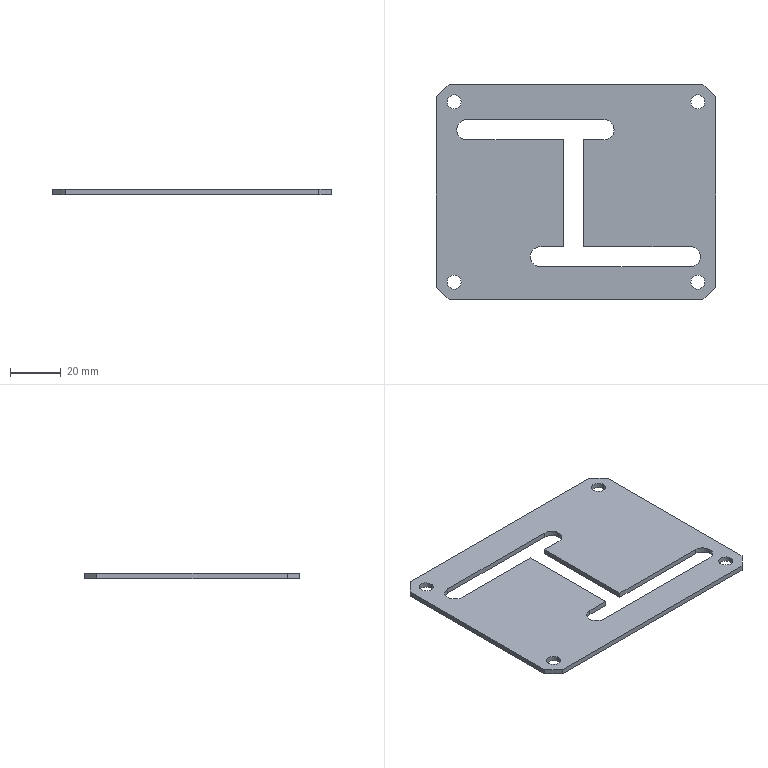Part | SolidWorks | features Cut 2, Extrusion 1 | 1 solid | 32 faces | box 110 x 85 x 2 mm | volume 15729 mm3 | plane 18 | cylinder 14 | commonest cylinder face diameters 5.5 x8 8 x5 8.02 x1
STEP:
#1=CARTESIAN_POINT('',(356.25,122.427,0.));
#2=VERTEX_POINT('',#1);
#3=CARTESIAN_POINT('',(361.75,122.427,0.));
#4=VERTEX_POINT('',#3);
#5=CARTESIAN_POINT('',(359.,122.427,0.));
#6=DIRECTION('',(0.,0.,1.));
#7=DIRECTION('',(1.,0.,0.));
#8=AXIS2_PLACEMENT_3D('',#5,#6,#7);
#9=CIRCLE('',#8,2.75);
#10=EDGE_CURVE('',#2,#4,#9,.T.);
#11=ORIENTED_EDGE('',*,*,#10,.F.);
#12=CARTESIAN_POINT('',(356.25,122.427,2.));
#13=VERTEX_POINT('',#12);
#14=CARTESIAN_POINT('',(356.25,122.427,0.));
#15=DIRECTION('',(0.,0.,1.));
#16=VECTOR('',#15,1000.);
#17=LINE('',#14,#16);
#18=EDGE_CURVE('',#2,#13,#17,.T.);
#19=ORIENTED_EDGE('',*,*,#18,.T.);
#20=CARTESIAN_POINT('',(361.75,122.427,2.));
#21=VERTEX_POINT('',#20);
#22=CARTESIAN_POINT('',(359.,122.427,2.));
#23=DIRECTION('',(0.,0.,1.));
#24=DIRECTION('',(1.,0.,0.));
#25=AXIS2_PLACEMENT_3D('',#22,#23,#24);
#26=CIRCLE('',#25,2.75);
#27=EDGE_CURVE('',#13,#21,#26,.T.);
#28=ORIENTED_EDGE('',*,*,#27,.T.);
#29=CARTESIAN_POINT('',(361.75,122.427,0.));
#30=DIRECTION('',(0.,0.,1.));
#31=VECTOR('',#30,1000.);
#32=LINE('',#29,#31);
#33=EDGE_CURVE('',#4,#21,#32,.T.);
#34=ORIENTED_EDGE('',*,*,#33,.F.);
#35=EDGE_LOOP('',(#11,#19,#28,#34));
#36=FACE_OUTER_BOUND('',#35,.T.);
#37=CARTESIAN_POINT('',(359.,122.427,0.));
#38=DIRECTION('',(0.,0.,1.));
#39=DIRECTION('',(1.,0.,0.));
#40=AXIS2_PLACEMENT_3D('',#37,#38,#39);
#41=CYLINDRICAL_SURFACE('',#40,2.75);
#42=ADVANCED_FACE('',(#36),#41,.F.);
#43=CARTESIAN_POINT('',(452.25,122.427,0.));
#44=VERTEX_POINT('',#43);
#45=CARTESIAN_POINT('',(457.75,122.427,0.));
#46=VERTEX_POINT('',#45);
#47=CARTESIAN_POINT('',(455.,122.427,0.));
#48=DIRECTION('',(0.,0.,1.));
#49=DIRECTION('',(1.,0.,0.));
#50=AXIS2_PLACEMENT_3D('',#47,#48,#49);
#51=CIRCLE('',#50,2.75);
#52=EDGE_CURVE('',#44,#46,#51,.T.);
#53=ORIENTED_EDGE('',*,*,#52,.F.);
#54=CARTESIAN_POINT('',(452.25,122.427,2.));
#55=VERTEX_POINT('',#54);
#56=CARTESIAN_POINT('',(452.25,122.427,0.));
#57=DIRECTION('',(0.,0.,1.));
#58=VECTOR('',#57,1000.);
#59=LINE('',#56,#58);
#60=EDGE_CURVE('',#44,#55,#59,.T.);
#61=ORIENTED_EDGE('',*,*,#60,.T.);
#62=CARTESIAN_POINT('',(457.75,122.427,2.));
#63=VERTEX_POINT('',#62);
#64=CARTESIAN_POINT('',(455.,122.427,2.));
#65=DIRECTION('',(0.,0.,1.));
#66=DIRECTION('',(1.,0.,0.));
#67=AXIS2_PLACEMENT_3D('',#64,#65,#66);
#68=CIRCLE('',#67,2.75);
#69=EDGE_CURVE('',#55,#63,#68,.T.);
#70=ORIENTED_EDGE('',*,*,#69,.T.);
#71=CARTESIAN_POINT('',(457.75,122.427,0.));
#72=DIRECTION('',(0.,0.,1.));
#73=VECTOR('',#72,1000.);
#74=LINE('',#71,#73);
#75=EDGE_CURVE('',#46,#63,#74,.T.);
#76=ORIENTED_EDGE('',*,*,#75,.F.);
#77=EDGE_LOOP('',(#53,#61,#70,#76));
#78=FACE_OUTER_BOUND('',#77,.T.);
#79=CARTESIAN_POINT('',(455.,122.427,0.));
#80=DIRECTION('',(0.,0.,1.));
#81=DIRECTION('',(1.,0.,0.));
#82=AXIS2_PLACEMENT_3D('',#79,#80,#81);
#83=CYLINDRICAL_SURFACE('',#82,2.75);
#84=ADVANCED_FACE('',(#78),#83,.F.);
#85=CARTESIAN_POINT('',(356.25,51.427,0.));
#86=VERTEX_POINT('',#85);
#87=CARTESIAN_POINT('',(361.75,51.427,0.));
#88=VERTEX_POINT('',#87);
#89=CARTESIAN_POINT('',(359.,51.427,0.));
#90=DIRECTION('',(0.,0.,1.));
#91=DIRECTION('',(1.,0.,0.));
#92=AXIS2_PLACEMENT_3D('',#89,#90,#91);
#93=CIRCLE('',#92,2.75);
#94=EDGE_CURVE('',#86,#88,#93,.T.);
#95=ORIENTED_EDGE('',*,*,#94,.F.);
#96=CARTESIAN_POINT('',(356.25,51.427,2.));
#97=VERTEX_POINT('',#96);
#98=CARTESIAN_POINT('',(356.25,51.427,0.));
#99=DIRECTION('',(0.,0.,1.));
#100=VECTOR('',#99,1000.);
#101=LINE('',#98,#100);
#102=EDGE_CURVE('',#86,#97,#101,.T.);
#103=ORIENTED_EDGE('',*,*,#102,.T.);
#104=CARTESIAN_POINT('',(361.75,51.427,2.));
#105=VERTEX_POINT('',#104);
#106=CARTESIAN_POINT('',(359.,51.427,2.));
#107=DIRECTION('',(0.,0.,1.));
#108=DIRECTION('',(1.,0.,0.));
#109=AXIS2_PLACEMENT_3D('',#106,#107,#108);
#110=CIRCLE('',#109,2.75);
#111=EDGE_CURVE('',#97,#105,#110,.T.);
#112=ORIENTED_EDGE('',*,*,#111,.T.);
#113=CARTESIAN_POINT('',(361.75,51.427,0.));
#114=DIRECTION('',(0.,0.,1.));
#115=VECTOR('',#114,1000.);
#116=LINE('',#113,#115);
#117=EDGE_CURVE('',#88,#105,#116,.T.);
#118=ORIENTED_EDGE('',*,*,#117,.F.);
#119=EDGE_LOOP('',(#95,#103,#112,#118));
#120=FACE_OUTER_BOUND('',#119,.T.);
#121=CARTESIAN_POINT('',(359.,51.427,0.));
#122=DIRECTION('',(0.,0.,1.));
#123=DIRECTION('',(1.,0.,0.));
#124=AXIS2_PLACEMENT_3D('',#121,#122,#123);
#125=CYLINDRICAL_SURFACE('',#124,2.75);
#126=ADVANCED_FACE('',(#120),#125,.F.);
#127=CARTESIAN_POINT('',(452.25,51.427,0.));
#128=VERTEX_POINT('',#127);
#129=CARTESIAN_POINT('',(457.75,51.427,0.));
#130=VERTEX_POINT('',#129);
#131=CARTESIAN_POINT('',(455.,51.427,0.));
#132=DIRECTION('',(0.,0.,1.));
#133=DIRECTION('',(1.,0.,0.));
#134=AXIS2_PLACEMENT_3D('',#131,#132,#133);
#135=CIRCLE('',#134,2.75);
#136=EDGE_CURVE('',#128,#130,#135,.T.);
#137=ORIENTED_EDGE('',*,*,#136,.F.);
#138=CARTESIAN_POINT('',(452.25,51.427,2.));
#139=VERTEX_POINT('',#138);
#140=CARTESIAN_POINT('',(452.25,51.427,0.));
#141=DIRECTION('',(0.,0.,1.));
#142=VECTOR('',#141,1000.);
#143=LINE('',#140,#142);
#144=EDGE_CURVE('',#128,#139,#143,.T.);
#145=ORIENTED_EDGE('',*,*,#144,.T.);
#146=CARTESIAN_POINT('',(457.75,51.427,2.));
#147=VERTEX_POINT('',#146);
#148=CARTESIAN_POINT('',(455.,51.427,2.));
#149=DIRECTION('',(0.,0.,1.));
#150=DIRECTION('',(1.,0.,0.));
#151=AXIS2_PLACEMENT_3D('',#148,#149,#150);
#152=CIRCLE('',#151,2.75);
#153=EDGE_CURVE('',#139,#147,#152,.T.);
#154=ORIENTED_EDGE('',*,*,#153,.T.);
#155=CARTESIAN_POINT('',(457.75,51.427,0.));
#156=DIRECTION('',(0.,0.,1.));
#157=VECTOR('',#156,1000.);
#158=LINE('',#155,#157);
#159=EDGE_CURVE('',#130,#147,#158,.T.);
#160=ORIENTED_EDGE('',*,*,#159,.F.);
#161=EDGE_LOOP('',(#137,#145,#154,#160));
#162=FACE_OUTER_BOUND('',#161,.T.);
#163=CARTESIAN_POINT('',(455.,51.427,0.));
#164=DIRECTION('',(0.,0.,1.));
#165=DIRECTION('',(1.,0.,0.));
#166=AXIS2_PLACEMENT_3D('',#163,#164,#165);
#167=CYLINDRICAL_SURFACE('',#166,2.75);
#168=ADVANCED_FACE('',(#162),#167,.F.);
#169=CARTESIAN_POINT('',(422.,111.427,0.));
#170=VERTEX_POINT('',#169);
#171=CARTESIAN_POINT('',(418.,115.427,0.));
#172=VERTEX_POINT('',#171);
#173=CARTESIAN_POINT('',(418.,111.427,0.));
#174=DIRECTION('',(0.,0.,1.));
#175=DIRECTION('',(1.,0.,0.));
#176=AXIS2_PLACEMENT_3D('',#173,#174,#175);
#177=CIRCLE('',#176,4.);
#178=EDGE_CURVE('',#170,#172,#177,.T.);
#179=ORIENTED_EDGE('',*,*,#178,.F.);
#180=CARTESIAN_POINT('',(422.,111.427,2.));
#181=VERTEX_POINT('',#180);
#182=CARTESIAN_POINT('',(422.,111.427,0.));
#183=DIRECTION('',(0.,0.,1.));
#184=VECTOR('',#183,1000.);
#185=LINE('',#182,#184);
#186=EDGE_CURVE('',#170,#181,#185,.T.);
#187=ORIENTED_EDGE('',*,*,#186,.T.);
#188=CARTESIAN_POINT('',(418.,115.427,2.));
#189=VERTEX_POINT('',#188);
#190=CARTESIAN_POINT('',(418.,111.427,2.));
#191=DIRECTION('',(0.,0.,1.));
#192=DIRECTION('',(1.,0.,0.));
#193=AXIS2_PLACEMENT_3D('',#190,#191,#192);
#194=CIRCLE('',#193,4.);
#195=EDGE_CURVE('',#181,#189,#194,.T.);
#196=ORIENTED_EDGE('',*,*,#195,.T.);
#197=CARTESIAN_POINT('',(418.,115.427,0.));
#198=DIRECTION('',(0.,0.,1.));
#199=VECTOR('',#198,1000.);
#200=LINE('',#197,#199);
#201=EDGE_CURVE('',#172,#189,#200,.T.);
#202=ORIENTED_EDGE('',*,*,#201,.F.);
#203=EDGE_LOOP('',(#179,#187,#196,#202));
#204=FACE_OUTER_BOUND('',#203,.T.);
#205=CARTESIAN_POINT('',(418.,111.427,0.));
#206=DIRECTION('',(0.,0.,1.));
#207=DIRECTION('',(1.,0.,0.));
#208=AXIS2_PLACEMENT_3D('',#205,#206,#207);
#209=CYLINDRICAL_SURFACE('',#208,4.);
#210=ADVANCED_FACE('',(#204),#209,.F.);
#211=CARTESIAN_POINT('',(456.,61.427,0.));
#212=VERTEX_POINT('',#211);
#213=CARTESIAN_POINT('',(452.,65.427,0.));
#214=VERTEX_POINT('',#213);
#215=CARTESIAN_POINT('',(452.,61.427,0.));
#216=DIRECTION('',(0.,0.,1.));
#217=DIRECTION('',(1.,0.,0.));
#218=AXIS2_PLACEMENT_3D('',#215,#216,#217);
#219=CIRCLE('',#218,4.);
#220=EDGE_CURVE('',#212,#214,#219,.T.);
#221=ORIENTED_EDGE('',*,*,#220,.F.);
#222=CARTESIAN_POINT('',(456.,61.427,2.));
#223=VERTEX_POINT('',#222);
#224=CARTESIAN_POINT('',(456.,61.427,0.));
#225=DIRECTION('',(0.,0.,1.));
#226=VECTOR('',#225,1000.);
#227=LINE('',#224,#226);
#228=EDGE_CURVE('',#212,#223,#227,.T.);
#229=ORIENTED_EDGE('',*,*,#228,.T.);
#230=CARTESIAN_POINT('',(452.,65.427,2.));
#231=VERTEX_POINT('',#230);
#232=CARTESIAN_POINT('',(452.,61.427,2.));
#233=DIRECTION('',(0.,0.,1.));
#234=DIRECTION('',(1.,0.,0.));
#235=AXIS2_PLACEMENT_3D('',#232,#233,#234);
#236=CIRCLE('',#235,4.);
#237=EDGE_CURVE('',#223,#231,#236,.T.);
#238=ORIENTED_EDGE('',*,*,#237,.T.);
#239=CARTESIAN_POINT('',(452.,65.427,0.));
#240=DIRECTION('',(0.,0.,1.));
#241=VECTOR('',#240,1000.);
#242=LINE('',#239,#241);
#243=EDGE_CURVE('',#214,#231,#242,.T.);
#244=ORIENTED_EDGE('',*,*,#243,.F.);
#245=EDGE_LOOP('',(#221,#229,#238,#244));
#246=FACE_OUTER_BOUND('',#245,.T.);
#247=CARTESIAN_POINT('',(452.,61.427,0.));
#248=DIRECTION('',(0.,0.,1.));
#249=DIRECTION('',(1.,0.,0.));
#250=AXIS2_PLACEMENT_3D('',#247,#248,#249);
#251=CYLINDRICAL_SURFACE('',#250,4.);
#252=ADVANCED_FACE('',(#246),#251,.F.);
#253=CARTESIAN_POINT('',(352.,49.427,0.));
#254=VERTEX_POINT('',#253);
#255=CARTESIAN_POINT('',(357.,44.427,0.));
#256=VERTEX_POINT('',#255);
#257=CARTESIAN_POINT('',(352.,49.427,0.));
#258=DIRECTION('',(0.7071,-0.7071,0.));
#259=VECTOR('',#258,1000.);
#260=LINE('',#257,#259);
#261=EDGE_CURVE('',#254,#256,#260,.T.);
#262=ORIENTED_EDGE('',*,*,#261,.T.);
#263=CARTESIAN_POINT('',(357.,44.427,2.));
#264=VERTEX_POINT('',#263);
#265=CARTESIAN_POINT('',(357.,44.427,2.));
#266=DIRECTION('',(0.,0.,-1.));
#267=VECTOR('',#266,1000.);
#268=LINE('',#265,#267);
#269=EDGE_CURVE('',#264,#256,#268,.T.);
#270=ORIENTED_EDGE('',*,*,#269,.F.);
#271=CARTESIAN_POINT('',(352.,49.427,2.));
#272=VERTEX_POINT('',#271);
#273=CARTESIAN_POINT('',(352.,49.427,2.));
#274=DIRECTION('',(0.7071,-0.7071,0.));
#275=VECTOR('',#274,1000.);
#276=LINE('',#273,#275);
#277=EDGE_CURVE('',#272,#264,#276,.T.);
#278=ORIENTED_EDGE('',*,*,#277,.F.);
#279=CARTESIAN_POINT('',(352.,49.427,2.));
#280=DIRECTION('',(0.,0.,-1.));
#281=VECTOR('',#280,1000.);
#282=LINE('',#279,#281);
#283=EDGE_CURVE('',#272,#254,#282,.T.);
#284=ORIENTED_EDGE('',*,*,#283,.T.);
#285=EDGE_LOOP('',(#262,#270,#278,#284));
#286=FACE_OUTER_BOUND('',#285,.T.);
#287=CARTESIAN_POINT('',(352.,49.427,2.));
#288=DIRECTION('',(0.7071,0.7071,0.));
#289=DIRECTION('',(-0.7071,0.7071,0.));
#290=AXIS2_PLACEMENT_3D('',#287,#288,#289);
#291=PLANE('',#290);
#292=ADVANCED_FACE('',(#286),#291,.F.);
#293=CARTESIAN_POINT('',(457.,44.427,0.));
#294=VERTEX_POINT('',#293);
#295=CARTESIAN_POINT('',(357.,44.427,0.));
#296=DIRECTION('',(1.,0.,0.));
#297=VECTOR('',#296,1000.);
#298=LINE('',#295,#297);
#299=EDGE_CURVE('',#256,#294,#298,.T.);
#300=ORIENTED_EDGE('',*,*,#299,.T.);
#301=CARTESIAN_POINT('',(457.,44.427,2.));
#302=VERTEX_POINT('',#301);
#303=CARTESIAN_POINT('',(457.,44.427,2.));
#304=DIRECTION('',(0.,0.,-1.));
#305=VECTOR('',#304,1000.);
#306=LINE('',#303,#305);
#307=EDGE_CURVE('',#302,#294,#306,.T.);
#308=ORIENTED_EDGE('',*,*,#307,.F.);
#309=CARTESIAN_POINT('',(357.,44.427,2.));
#310=DIRECTION('',(1.,0.,0.));
#311=VECTOR('',#310,1000.);
#312=LINE('',#309,#311);
#313=EDGE_CURVE('',#264,#302,#312,.T.);
#314=ORIENTED_EDGE('',*,*,#313,.F.);
#315=ORIENTED_EDGE('',*,*,#269,.T.);
#316=EDGE_LOOP('',(#300,#308,#314,#315));
#317=FACE_OUTER_BOUND('',#316,.T.);
#318=CARTESIAN_POINT('',(357.,44.427,2.));
#319=DIRECTION('',(0.,1.,0.));
#320=DIRECTION('',(-1.,0.,0.));
#321=AXIS2_PLACEMENT_3D('',#318,#319,#320);
#322=PLANE('',#321);
#323=ADVANCED_FACE('',(#317),#322,.F.);
#324=CARTESIAN_POINT('',(462.,49.427,0.));
#325=VERTEX_POINT('',#324);
#326=CARTESIAN_POINT('',(457.,44.427,0.));
#327=DIRECTION('',(0.7071,0.7071,0.));
#328=VECTOR('',#327,1000.);
#329=LINE('',#326,#328);
#330=EDGE_CURVE('',#294,#325,#329,.T.);
#331=ORIENTED_EDGE('',*,*,#330,.T.);
#332=CARTESIAN_POINT('',(462.,49.427,2.));
#333=VERTEX_POINT('',#332);
#334=CARTESIAN_POINT('',(462.,49.427,2.));
#335=DIRECTION('',(0.,0.,-1.));
#336=VECTOR('',#335,1000.);
#337=LINE('',#334,#336);
#338=EDGE_CURVE('',#333,#325,#337,.T.);
#339=ORIENTED_EDGE('',*,*,#338,.F.);
#340=CARTESIAN_POINT('',(457.,44.427,2.));
#341=DIRECTION('',(0.7071,0.7071,0.));
#342=VECTOR('',#341,1000.);
#343=LINE('',#340,#342);
#344=EDGE_CURVE('',#302,#333,#343,.T.);
#345=ORIENTED_EDGE('',*,*,#344,.F.);
#346=ORIENTED_EDGE('',*,*,#307,.T.);
#347=EDGE_LOOP('',(#331,#339,#345,#346));
#348=FACE_OUTER_BOUND('',#347,.T.);
#349=CARTESIAN_POINT('',(457.,44.427,2.));
#350=DIRECTION('',(-0.7071,0.7071,0.));
#351=DIRECTION('',(-0.7071,-0.7071,0.));
#352=AXIS2_PLACEMENT_3D('',#349,#350,#351);
#353=PLANE('',#352);
#354=ADVANCED_FACE('',(#348),#353,.F.);
#355=CARTESIAN_POINT('',(462.,124.427,0.));
#356=VERTEX_POINT('',#355);
#357=CARTESIAN_POINT('',(462.,49.427,0.));
#358=DIRECTION('',(0.,1.,0.));
#359=VECTOR('',#358,1000.);
#360=LINE('',#357,#359);
#361=EDGE_CURVE('',#325,#356,#360,.T.);
#362=ORIENTED_EDGE('',*,*,#361,.T.);
#363=CARTESIAN_POINT('',(462.,124.427,2.));
#364=VERTEX_POINT('',#363);
#365=CARTESIAN_POINT('',(462.,124.427,2.));
#366=DIRECTION('',(0.,0.,-1.));
#367=VECTOR('',#366,1000.);
#368=LINE('',#365,#367);
#369=EDGE_CURVE('',#364,#356,#368,.T.);
#370=ORIENTED_EDGE('',*,*,#369,.F.);
#371=CARTESIAN_POINT('',(462.,49.427,2.));
#372=DIRECTION('',(0.,1.,0.));
#373=VECTOR('',#372,1000.);
#374=LINE('',#371,#373);
#375=EDGE_CURVE('',#333,#364,#374,.T.);
#376=ORIENTED_EDGE('',*,*,#375,.F.);
#377=ORIENTED_EDGE('',*,*,#338,.T.);
#378=EDGE_LOOP('',(#362,#370,#376,#377));
#379=FACE_OUTER_BOUND('',#378,.T.);
#380=CARTESIAN_POINT('',(462.,49.427,2.));
#381=DIRECTION('',(-1.,0.,0.));
#382=DIRECTION('',(0.,0.,1.));
#383=AXIS2_PLACEMENT_3D('',#380,#381,#382);
#384=PLANE('',#383);
#385=ADVANCED_FACE('',(#379),#384,.F.);
#386=CARTESIAN_POINT('',(457.,129.427,0.));
#387=VERTEX_POINT('',#386);
#388=CARTESIAN_POINT('',(462.,124.427,0.));
#389=DIRECTION('',(-0.7071,0.7071,0.));
#390=VECTOR('',#389,1000.);
#391=LINE('',#388,#390);
#392=EDGE_CURVE('',#356,#387,#391,.T.);
#393=ORIENTED_EDGE('',*,*,#392,.T.);
#394=CARTESIAN_POINT('',(457.,129.427,2.));
#395=VERTEX_POINT('',#394);
#396=CARTESIAN_POINT('',(457.,129.427,2.));
#397=DIRECTION('',(0.,0.,-1.));
#398=VECTOR('',#397,1000.);
#399=LINE('',#396,#398);
#400=EDGE_CURVE('',#395,#387,#399,.T.);
#401=ORIENTED_EDGE('',*,*,#400,.F.);
#402=CARTESIAN_POINT('',(462.,124.427,2.));
#403=DIRECTION('',(-0.7071,0.7071,0.));
#404=VECTOR('',#403,1000.);
#405=LINE('',#402,#404);
#406=EDGE_CURVE('',#364,#395,#405,.T.);
#407=ORIENTED_EDGE('',*,*,#406,.F.);
#408=ORIENTED_EDGE('',*,*,#369,.T.);
#409=EDGE_LOOP('',(#393,#401,#407,#408));
#410=FACE_OUTER_BOUND('',#409,.T.);
#411=CARTESIAN_POINT('',(462.,124.427,2.));
#412=DIRECTION('',(-0.7071,-0.7071,0.));
#413=DIRECTION('',(0.7071,-0.7071,0.));
#414=AXIS2_PLACEMENT_3D('',#411,#412,#413);
#415=PLANE('',#414);
#416=ADVANCED_FACE('',(#410),#415,.F.);
#417=CARTESIAN_POINT('',(357.,129.427,0.));
#418=VERTEX_POINT('',#417);
#419=CARTESIAN_POINT('',(457.,129.427,0.));
#420=DIRECTION('',(-1.,0.,0.));
#421=VECTOR('',#420,1000.);
#422=LINE('',#419,#421);
#423=EDGE_CURVE('',#387,#418,#422,.T.);
#424=ORIENTED_EDGE('',*,*,#423,.T.);
#425=CARTESIAN_POINT('',(357.,129.427,2.));
#426=VERTEX_POINT('',#425);
#427=CARTESIAN_POINT('',(357.,129.427,2.));
#428=DIRECTION('',(0.,0.,-1.));
#429=VECTOR('',#428,1000.);
#430=LINE('',#427,#429);
#431=EDGE_CURVE('',#426,#418,#430,.T.);
#432=ORIENTED_EDGE('',*,*,#431,.F.);
#433=CARTESIAN_POINT('',(457.,129.427,2.));
#434=DIRECTION('',(-1.,0.,0.));
#435=VECTOR('',#434,1000.);
#436=LINE('',#433,#435);
#437=EDGE_CURVE('',#395,#426,#436,.T.);
#438=ORIENTED_EDGE('',*,*,#437,.F.);
#439=ORIENTED_EDGE('',*,*,#400,.T.);
#440=EDGE_LOOP('',(#424,#432,#438,#439));
#441=FACE_OUTER_BOUND('',#440,.T.);
#442=CARTESIAN_POINT('',(457.,129.427,2.));
#443=DIRECTION('',(0.,-1.,0.));
#444=DIRECTION('',(0.,0.,-1.));
#445=AXIS2_PLACEMENT_3D('',#442,#443,#444);
#446=PLANE('',#445);
#447=ADVANCED_FACE('',(#441),#446,.F.);
#448=CARTESIAN_POINT('',(352.,124.427,0.));
#449=VERTEX_POINT('',#448);
#450=CARTESIAN_POINT('',(357.,129.427,0.));
#451=DIRECTION('',(-0.7071,-0.7071,0.));
#452=VECTOR('',#451,1000.);
#453=LINE('',#450,#452);
#454=EDGE_CURVE('',#418,#449,#453,.T.);
#455=ORIENTED_EDGE('',*,*,#454,.T.);
#456=CARTESIAN_POINT('',(352.,124.427,2.));
#457=VERTEX_POINT('',#456);
#458=CARTESIAN_POINT('',(352.,124.427,2.));
#459=DIRECTION('',(0.,0.,-1.));
#460=VECTOR('',#459,1000.);
#461=LINE('',#458,#460);
#462=EDGE_CURVE('',#457,#449,#461,.T.);
#463=ORIENTED_EDGE('',*,*,#462,.F.);
#464=CARTESIAN_POINT('',(357.,129.427,2.));
#465=DIRECTION('',(-0.7071,-0.7071,0.));
#466=VECTOR('',#465,1000.);
#467=LINE('',#464,#466);
#468=EDGE_CURVE('',#426,#457,#467,.T.);
#469=ORIENTED_EDGE('',*,*,#468,.F.);
#470=ORIENTED_EDGE('',*,*,#431,.T.);
#471=EDGE_LOOP('',(#455,#463,#469,#470));
#472=FACE_OUTER_BOUND('',#471,.T.);
#473=CARTESIAN_POINT('',(357.,129.427,2.));
#474=DIRECTION('',(0.7071,-0.7071,0.));
#475=DIRECTION('',(0.7071,0.7071,0.));
#476=AXIS2_PLACEMENT_3D('',#473,#474,#475);
#477=PLANE('',#476);
#478=ADVANCED_FACE('',(#472),#477,.F.);
#479=CARTESIAN_POINT('',(352.,124.427,0.));
#480=DIRECTION('',(0.,-1.,0.));
#481=VECTOR('',#480,1000.);
#482=LINE('',#479,#481);
#483=EDGE_CURVE('',#449,#254,#482,.T.);
#484=ORIENTED_EDGE('',*,*,#483,.T.);
#485=ORIENTED_EDGE('',*,*,#283,.F.);
#486=CARTESIAN_POINT('',(352.,124.427,2.));
#487=DIRECTION('',(0.,-1.,0.));
#488=VECTOR('',#487,1000.);
#489=LINE('',#486,#488);
#490=EDGE_CURVE('',#457,#272,#489,.T.);
#491=ORIENTED_EDGE('',*,*,#490,.F.);
#492=ORIENTED_EDGE('',*,*,#462,.T.);
#493=EDGE_LOOP('',(#484,#485,#491,#492));
#494=FACE_OUTER_BOUND('',#493,.T.);
#495=CARTESIAN_POINT('',(352.,124.427,2.));
#496=DIRECTION('',(1.,0.,0.));
#497=DIRECTION('',(0.,1.,0.));
#498=AXIS2_PLACEMENT_3D('',#495,#496,#497);
#499=PLANE('',#498);
#500=ADVANCED_FACE('',(#494),#499,.F.);
#501=CARTESIAN_POINT('',(359.,122.427,2.));
#502=DIRECTION('',(0.,0.,1.));
#503=DIRECTION('',(1.,0.,0.));
#504=AXIS2_PLACEMENT_3D('',#501,#502,#503);
#505=CIRCLE('',#504,2.75);
#506=EDGE_CURVE('',#21,#13,#505,.T.);
#507=ORIENTED_EDGE('',*,*,#506,.F.);
#508=ORIENTED_EDGE('',*,*,#27,.F.);
#509=EDGE_LOOP('',(#507,#508));
#510=FACE_BOUND('',#509,.T.);
#511=CARTESIAN_POINT('',(455.,122.427,2.));
#512=DIRECTION('',(0.,0.,1.));
#513=DIRECTION('',(1.,0.,0.));
#514=AXIS2_PLACEMENT_3D('',#511,#512,#513);
#515=CIRCLE('',#514,2.75);
#516=EDGE_CURVE('',#63,#55,#515,.T.);
#517=ORIENTED_EDGE('',*,*,#516,.F.);
#518=ORIENTED_EDGE('',*,*,#69,.F.);
#519=EDGE_LOOP('',(#517,#518));
#520=FACE_BOUND('',#519,.T.);
#521=CARTESIAN_POINT('',(359.,51.427,2.));
#522=DIRECTION('',(0.,0.,1.));
#523=DIRECTION('',(1.,0.,0.));
#524=AXIS2_PLACEMENT_3D('',#521,#522,#523);
#525=CIRCLE('',#524,2.75);
#526=EDGE_CURVE('',#105,#97,#525,.T.);
#527=ORIENTED_EDGE('',*,*,#526,.F.);
#528=ORIENTED_EDGE('',*,*,#111,.F.);
#529=EDGE_LOOP('',(#527,#528));
#530=FACE_BOUND('',#529,.T.);
#531=CARTESIAN_POINT('',(455.,51.427,2.));
#532=DIRECTION('',(0.,0.,1.));
#533=DIRECTION('',(1.,0.,0.));
#534=AXIS2_PLACEMENT_3D('',#531,#532,#533);
#535=CIRCLE('',#534,2.75);
#536=EDGE_CURVE('',#147,#139,#535,.T.);
#537=ORIENTED_EDGE('',*,*,#536,.F.);
#538=ORIENTED_EDGE('',*,*,#153,.F.);
#539=EDGE_LOOP('',(#537,#538));
#540=FACE_BOUND('',#539,.T.);
#541=CARTESIAN_POINT('',(452.,57.427,2.));
#542=VERTEX_POINT('',#541);
#543=CARTESIAN_POINT('',(452.,61.427,2.));
#544=DIRECTION('',(0.,0.,1.));
#545=DIRECTION('',(1.,0.,0.));
#546=AXIS2_PLACEMENT_3D('',#543,#544,#545);
#547=CIRCLE('',#546,4.);
#548=EDGE_CURVE('',#542,#223,#547,.T.);
#549=ORIENTED_EDGE('',*,*,#548,.F.);
#550=CARTESIAN_POINT('',(392.719,57.427,2.));
#551=VERTEX_POINT('',#550);
#552=CARTESIAN_POINT('',(452.,57.427,2.));
#553=DIRECTION('',(1.,0.,0.));
#554=VECTOR('',#553,1000.);
#555=LINE('',#552,#554);
#556=EDGE_CURVE('',#551,#542,#555,.T.);
#557=ORIENTED_EDGE('',*,*,#556,.F.);
#558=CARTESIAN_POINT('',(393.281,65.427,2.));
#559=VERTEX_POINT('',#558);
#560=CARTESIAN_POINT('',(393.,61.427,2.));
#561=DIRECTION('',(0.,0.,1.));
#562=DIRECTION('',(1.,0.,0.));
#563=AXIS2_PLACEMENT_3D('',#560,#561,#562);
#564=CIRCLE('',#563,4.01);
#565=EDGE_CURVE('',#559,#551,#564,.T.);
#566=ORIENTED_EDGE('',*,*,#565,.F.);
#567=CARTESIAN_POINT('',(402.,65.427,2.));
#568=VERTEX_POINT('',#567);
#569=CARTESIAN_POINT('',(402.,65.427,2.));
#570=DIRECTION('',(-1.,0.,0.));
#571=VECTOR('',#570,1000.);
#572=LINE('',#569,#571);
#573=EDGE_CURVE('',#568,#559,#572,.T.);
#574=ORIENTED_EDGE('',*,*,#573,.F.);
#575=CARTESIAN_POINT('',(402.,107.427,2.));
#576=VERTEX_POINT('',#575);
#577=CARTESIAN_POINT('',(402.,65.427,2.));
#578=DIRECTION('',(0.,-1.,0.));
#579=VECTOR('',#578,1000.);
#580=LINE('',#577,#579);
#581=EDGE_CURVE('',#576,#568,#580,.T.);
#582=ORIENTED_EDGE('',*,*,#581,.F.);
#583=CARTESIAN_POINT('',(364.,107.427,2.));
#584=VERTEX_POINT('',#583);
#585=CARTESIAN_POINT('',(402.,107.427,2.));
#586=DIRECTION('',(1.,0.,0.));
#587=VECTOR('',#586,1000.);
#588=LINE('',#585,#587);
#589=EDGE_CURVE('',#584,#576,#588,.T.);
#590=ORIENTED_EDGE('',*,*,#589,.F.);
#591=CARTESIAN_POINT('',(364.,115.427,2.));
#592=VERTEX_POINT('',#591);
#593=CARTESIAN_POINT('',(364.,111.427,2.));
#594=DIRECTION('',(0.,0.,1.));
#595=DIRECTION('',(1.,0.,0.));
#596=AXIS2_PLACEMENT_3D('',#593,#594,#595);
#597=CIRCLE('',#596,4.);
#598=EDGE_CURVE('',#592,#584,#597,.T.);
#599=ORIENTED_EDGE('',*,*,#598,.F.);
#600=CARTESIAN_POINT('',(418.,115.427,2.));
#601=DIRECTION('',(-1.,0.,0.));
#602=VECTOR('',#601,1000.);
#603=LINE('',#600,#602);
#604=EDGE_CURVE('',#189,#592,#603,.T.);
#605=ORIENTED_EDGE('',*,*,#604,.F.);
#606=ORIENTED_EDGE('',*,*,#195,.F.);
#607=CARTESIAN_POINT('',(418.,107.427,2.));
#608=VERTEX_POINT('',#607);
#609=CARTESIAN_POINT('',(418.,111.427,2.));
#610=DIRECTION('',(0.,0.,1.));
#611=DIRECTION('',(1.,0.,0.));
#612=AXIS2_PLACEMENT_3D('',#609,#610,#611);
#613=CIRCLE('',#612,4.);
#614=EDGE_CURVE('',#608,#181,#613,.T.);
#615=ORIENTED_EDGE('',*,*,#614,.F.);
#616=CARTESIAN_POINT('',(410.,107.427,2.));
#617=VERTEX_POINT('',#616);
#618=CARTESIAN_POINT('',(418.,107.427,2.));
#619=DIRECTION('',(1.,0.,0.));
#620=VECTOR('',#619,1000.);
#621=LINE('',#618,#620);
#622=EDGE_CURVE('',#617,#608,#621,.T.);
#623=ORIENTED_EDGE('',*,*,#622,.F.);
#624=CARTESIAN_POINT('',(410.,65.427,2.));
#625=VERTEX_POINT('',#624);
#626=CARTESIAN_POINT('',(410.,65.427,2.));
#627=DIRECTION('',(0.,1.,0.));
#628=VECTOR('',#627,1000.);
#629=LINE('',#626,#628);
#630=EDGE_CURVE('',#625,#617,#629,.T.);
#631=ORIENTED_EDGE('',*,*,#630,.F.);
#632=CARTESIAN_POINT('',(452.,65.427,2.));
#633=DIRECTION('',(-1.,0.,0.));
#634=VECTOR('',#633,1000.);
#635=LINE('',#632,#634);
#636=EDGE_CURVE('',#231,#625,#635,.T.);
#637=ORIENTED_EDGE('',*,*,#636,.F.);
#638=ORIENTED_EDGE('',*,*,#237,.F.);
#639=EDGE_LOOP('',(#549,#557,#566,#574,#582,#590,#599,#605,#606,#615,#623,#631,#637,#638));
#640=FACE_BOUND('',#639,.T.);
#641=ORIENTED_EDGE('',*,*,#277,.T.);
#642=ORIENTED_EDGE('',*,*,#313,.T.);
#643=ORIENTED_EDGE('',*,*,#344,.T.);
#644=ORIENTED_EDGE('',*,*,#375,.T.);
#645=ORIENTED_EDGE('',*,*,#406,.T.);
#646=ORIENTED_EDGE('',*,*,#437,.T.);
#647=ORIENTED_EDGE('',*,*,#468,.T.);
#648=ORIENTED_EDGE('',*,*,#490,.T.);
#649=EDGE_LOOP('',(#641,#642,#643,#644,#645,#646,#647,#648));
#650=FACE_OUTER_BOUND('',#649,.T.);
#651=CARTESIAN_POINT('',(0.,0.,2.));
#652=DIRECTION('',(0.,0.,1.));
#653=DIRECTION('',(1.,0.,0.));
#654=AXIS2_PLACEMENT_3D('',#651,#652,#653);
#655=PLANE('',#654);
#656=ADVANCED_FACE('',(#510,#520,#530,#540,#640,#650),#655,.T.);
#657=CARTESIAN_POINT('',(359.,122.427,0.));
#658=DIRECTION('',(0.,0.,1.));
#659=DIRECTION('',(1.,0.,0.));
#660=AXIS2_PLACEMENT_3D('',#657,#658,#659);
#661=CIRCLE('',#660,2.75);
#662=EDGE_CURVE('',#4,#2,#661,.T.);
#663=ORIENTED_EDGE('',*,*,#662,.T.);
#664=ORIENTED_EDGE('',*,*,#10,.T.);
#665=EDGE_LOOP('',(#663,#664));
#666=FACE_BOUND('',#665,.T.);
#667=CARTESIAN_POINT('',(455.,122.427,0.));
#668=DIRECTION('',(0.,0.,1.));
#669=DIRECTION('',(1.,0.,0.));
#670=AXIS2_PLACEMENT_3D('',#667,#668,#669);
#671=CIRCLE('',#670,2.75);
#672=EDGE_CURVE('',#46,#44,#671,.T.);
#673=ORIENTED_EDGE('',*,*,#672,.T.);
#674=ORIENTED_EDGE('',*,*,#52,.T.);
#675=EDGE_LOOP('',(#673,#674));
#676=FACE_BOUND('',#675,.T.);
#677=CARTESIAN_POINT('',(359.,51.427,0.));
#678=DIRECTION('',(0.,0.,1.));
#679=DIRECTION('',(1.,0.,0.));
#680=AXIS2_PLACEMENT_3D('',#677,#678,#679);
#681=CIRCLE('',#680,2.75);
#682=EDGE_CURVE('',#88,#86,#681,.T.);
#683=ORIENTED_EDGE('',*,*,#682,.T.);
#684=ORIENTED_EDGE('',*,*,#94,.T.);
#685=EDGE_LOOP('',(#683,#684));
#686=FACE_BOUND('',#685,.T.);
#687=CARTESIAN_POINT('',(455.,51.427,0.));
#688=DIRECTION('',(0.,0.,1.));
#689=DIRECTION('',(1.,0.,0.));
#690=AXIS2_PLACEMENT_3D('',#687,#688,#689);
#691=CIRCLE('',#690,2.75);
#692=EDGE_CURVE('',#130,#128,#691,.T.);
#693=ORIENTED_EDGE('',*,*,#692,.T.);
#694=ORIENTED_EDGE('',*,*,#136,.T.);
#695=EDGE_LOOP('',(#693,#694));
#696=FACE_BOUND('',#695,.T.);
#697=CARTESIAN_POINT('',(392.719,57.427,0.));
#698=VERTEX_POINT('',#697);
#699=CARTESIAN_POINT('',(452.,57.427,0.));
#700=VERTEX_POINT('',#699);
#701=CARTESIAN_POINT('',(452.,57.427,0.));
#702=DIRECTION('',(1.,0.,0.));
#703=VECTOR('',#702,1000.);
#704=LINE('',#701,#703);
#705=EDGE_CURVE('',#698,#700,#704,.T.);
#706=ORIENTED_EDGE('',*,*,#705,.T.);
#707=CARTESIAN_POINT('',(452.,61.427,0.));
#708=DIRECTION('',(0.,0.,1.));
#709=DIRECTION('',(1.,0.,0.));
#710=AXIS2_PLACEMENT_3D('',#707,#708,#709);
#711=CIRCLE('',#710,4.);
#712=EDGE_CURVE('',#700,#212,#711,.T.);
#713=ORIENTED_EDGE('',*,*,#712,.T.);
#714=ORIENTED_EDGE('',*,*,#220,.T.);
#715=CARTESIAN_POINT('',(410.,65.427,0.));
#716=VERTEX_POINT('',#715);
#717=CARTESIAN_POINT('',(452.,65.427,0.));
#718=DIRECTION('',(-1.,0.,0.));
#719=VECTOR('',#718,1000.);
#720=LINE('',#717,#719);
#721=EDGE_CURVE('',#214,#716,#720,.T.);
#722=ORIENTED_EDGE('',*,*,#721,.T.);
#723=CARTESIAN_POINT('',(410.,107.427,0.));
#724=VERTEX_POINT('',#723);
#725=CARTESIAN_POINT('',(410.,65.427,0.));
#726=DIRECTION('',(0.,1.,0.));
#727=VECTOR('',#726,1000.);
#728=LINE('',#725,#727);
#729=EDGE_CURVE('',#716,#724,#728,.T.);
#730=ORIENTED_EDGE('',*,*,#729,.T.);
#731=CARTESIAN_POINT('',(418.,107.427,0.));
#732=VERTEX_POINT('',#731);
#733=CARTESIAN_POINT('',(418.,107.427,0.));
#734=DIRECTION('',(1.,0.,0.));
#735=VECTOR('',#734,1000.);
#736=LINE('',#733,#735);
#737=EDGE_CURVE('',#724,#732,#736,.T.);
#738=ORIENTED_EDGE('',*,*,#737,.T.);
#739=CARTESIAN_POINT('',(418.,111.427,0.));
#740=DIRECTION('',(0.,0.,1.));
#741=DIRECTION('',(1.,0.,0.));
#742=AXIS2_PLACEMENT_3D('',#739,#740,#741);
#743=CIRCLE('',#742,4.);
#744=EDGE_CURVE('',#732,#170,#743,.T.);
#745=ORIENTED_EDGE('',*,*,#744,.T.);
#746=ORIENTED_EDGE('',*,*,#178,.T.);
#747=CARTESIAN_POINT('',(364.,115.427,0.));
#748=VERTEX_POINT('',#747);
#749=CARTESIAN_POINT('',(418.,115.427,0.));
#750=DIRECTION('',(-1.,0.,0.));
#751=VECTOR('',#750,1000.);
#752=LINE('',#749,#751);
#753=EDGE_CURVE('',#172,#748,#752,.T.);
#754=ORIENTED_EDGE('',*,*,#753,.T.);
#755=CARTESIAN_POINT('',(364.,107.427,0.));
#756=VERTEX_POINT('',#755);
#757=CARTESIAN_POINT('',(364.,111.427,0.));
#758=DIRECTION('',(0.,0.,1.));
#759=DIRECTION('',(1.,0.,0.));
#760=AXIS2_PLACEMENT_3D('',#757,#758,#759);
#761=CIRCLE('',#760,4.);
#762=EDGE_CURVE('',#748,#756,#761,.T.);
#763=ORIENTED_EDGE('',*,*,#762,.T.);
#764=CARTESIAN_POINT('',(402.,107.427,0.));
#765=VERTEX_POINT('',#764);
#766=CARTESIAN_POINT('',(402.,107.427,0.));
#767=DIRECTION('',(1.,0.,0.));
#768=VECTOR('',#767,1000.);
#769=LINE('',#766,#768);
#770=EDGE_CURVE('',#756,#765,#769,.T.);
#771=ORIENTED_EDGE('',*,*,#770,.T.);
#772=CARTESIAN_POINT('',(402.,65.427,0.));
#773=VERTEX_POINT('',#772);
#774=CARTESIAN_POINT('',(402.,65.427,0.));
#775=DIRECTION('',(0.,-1.,0.));
#776=VECTOR('',#775,1000.);
#777=LINE('',#774,#776);
#778=EDGE_CURVE('',#765,#773,#777,.T.);
#779=ORIENTED_EDGE('',*,*,#778,.T.);
#780=CARTESIAN_POINT('',(393.281,65.427,0.));
#781=VERTEX_POINT('',#780);
#782=CARTESIAN_POINT('',(402.,65.427,0.));
#783=DIRECTION('',(-1.,0.,0.));
#784=VECTOR('',#783,1000.);
#785=LINE('',#782,#784);
#786=EDGE_CURVE('',#773,#781,#785,.T.);
#787=ORIENTED_EDGE('',*,*,#786,.T.);
#788=CARTESIAN_POINT('',(393.,61.427,0.));
#789=DIRECTION('',(0.,0.,1.));
#790=DIRECTION('',(1.,0.,0.));
#791=AXIS2_PLACEMENT_3D('',#788,#789,#790);
#792=CIRCLE('',#791,4.01);
#793=EDGE_CURVE('',#781,#698,#792,.T.);
#794=ORIENTED_EDGE('',*,*,#793,.T.);
#795=EDGE_LOOP('',(#706,#713,#714,#722,#730,#738,#745,#746,#754,#763,#771,#779,#787,#794));
#796=FACE_BOUND('',#795,.T.);
#797=ORIENTED_EDGE('',*,*,#261,.F.);
#798=ORIENTED_EDGE('',*,*,#483,.F.);
#799=ORIENTED_EDGE('',*,*,#454,.F.);
#800=ORIENTED_EDGE('',*,*,#423,.F.);
#801=ORIENTED_EDGE('',*,*,#392,.F.);
#802=ORIENTED_EDGE('',*,*,#361,.F.);
#803=ORIENTED_EDGE('',*,*,#330,.F.);
#804=ORIENTED_EDGE('',*,*,#299,.F.);
#805=EDGE_LOOP('',(#797,#798,#799,#800,#801,#802,#803,#804));
#806=FACE_OUTER_BOUND('',#805,.T.);
#807=CARTESIAN_POINT('',(0.,0.,0.));
#808=DIRECTION('',(0.,0.,1.));
#809=DIRECTION('',(1.,0.,0.));
#810=AXIS2_PLACEMENT_3D('',#807,#808,#809);
#811=PLANE('',#810);
#812=ADVANCED_FACE('',(#666,#676,#686,#696,#796,#806),#811,.F.);
#813=ORIENTED_EDGE('',*,*,#228,.F.);
#814=ORIENTED_EDGE('',*,*,#712,.F.);
#815=CARTESIAN_POINT('',(452.,57.427,0.));
#816=DIRECTION('',(0.,0.,1.));
#817=VECTOR('',#816,1000.);
#818=LINE('',#815,#817);
#819=EDGE_CURVE('',#700,#542,#818,.T.);
#820=ORIENTED_EDGE('',*,*,#819,.T.);
#821=ORIENTED_EDGE('',*,*,#548,.T.);
#822=EDGE_LOOP('',(#813,#814,#820,#821));
#823=FACE_OUTER_BOUND('',#822,.T.);
#824=CARTESIAN_POINT('',(452.,61.427,0.));
#825=DIRECTION('',(0.,0.,1.));
#826=DIRECTION('',(1.,0.,0.));
#827=AXIS2_PLACEMENT_3D('',#824,#825,#826);
#828=CYLINDRICAL_SURFACE('',#827,4.);
#829=ADVANCED_FACE('',(#823),#828,.F.);
#830=ORIENTED_EDGE('',*,*,#556,.T.);
#831=ORIENTED_EDGE('',*,*,#819,.F.);
#832=ORIENTED_EDGE('',*,*,#705,.F.);
#833=CARTESIAN_POINT('',(392.719,57.427,0.));
#834=DIRECTION('',(0.,0.,1.));
#835=VECTOR('',#834,1000.);
#836=LINE('',#833,#835);
#837=EDGE_CURVE('',#698,#551,#836,.T.);
#838=ORIENTED_EDGE('',*,*,#837,.T.);
#839=EDGE_LOOP('',(#830,#831,#832,#838));
#840=FACE_OUTER_BOUND('',#839,.T.);
#841=CARTESIAN_POINT('',(452.,57.427,0.));
#842=DIRECTION('',(0.,-1.,0.));
#843=DIRECTION('',(1.,0.,0.));
#844=AXIS2_PLACEMENT_3D('',#841,#842,#843);
#845=PLANE('',#844);
#846=ADVANCED_FACE('',(#840),#845,.F.);
#847=ORIENTED_EDGE('',*,*,#565,.T.);
#848=ORIENTED_EDGE('',*,*,#837,.F.);
#849=ORIENTED_EDGE('',*,*,#793,.F.);
#850=CARTESIAN_POINT('',(393.281,65.427,0.));
#851=DIRECTION('',(0.,0.,1.));
#852=VECTOR('',#851,1000.);
#853=LINE('',#850,#852);
#854=EDGE_CURVE('',#781,#559,#853,.T.);
#855=ORIENTED_EDGE('',*,*,#854,.T.);
#856=EDGE_LOOP('',(#847,#848,#849,#855));
#857=FACE_OUTER_BOUND('',#856,.T.);
#858=CARTESIAN_POINT('',(393.,61.427,0.));
#859=DIRECTION('',(0.,0.,1.));
#860=DIRECTION('',(1.,0.,0.));
#861=AXIS2_PLACEMENT_3D('',#858,#859,#860);
#862=CYLINDRICAL_SURFACE('',#861,4.01);
#863=ADVANCED_FACE('',(#857),#862,.F.);
#864=ORIENTED_EDGE('',*,*,#573,.T.);
#865=ORIENTED_EDGE('',*,*,#854,.F.);
#866=ORIENTED_EDGE('',*,*,#786,.F.);
#867=CARTESIAN_POINT('',(402.,65.427,0.));
#868=DIRECTION('',(0.,0.,1.));
#869=VECTOR('',#868,1000.);
#870=LINE('',#867,#869);
#871=EDGE_CURVE('',#773,#568,#870,.T.);
#872=ORIENTED_EDGE('',*,*,#871,.T.);
#873=EDGE_LOOP('',(#864,#865,#866,#872));
#874=FACE_OUTER_BOUND('',#873,.T.);
#875=CARTESIAN_POINT('',(402.,65.427,0.));
#876=DIRECTION('',(0.,1.,0.));
#877=DIRECTION('',(-1.,0.,0.));
#878=AXIS2_PLACEMENT_3D('',#875,#876,#877);
#879=PLANE('',#878);
#880=ADVANCED_FACE('',(#874),#879,.F.);
#881=ORIENTED_EDGE('',*,*,#581,.T.);
#882=ORIENTED_EDGE('',*,*,#871,.F.);
#883=ORIENTED_EDGE('',*,*,#778,.F.);
#884=CARTESIAN_POINT('',(402.,107.427,0.));
#885=DIRECTION('',(0.,0.,1.));
#886=VECTOR('',#885,1000.);
#887=LINE('',#884,#886);
#888=EDGE_CURVE('',#765,#576,#887,.T.);
#889=ORIENTED_EDGE('',*,*,#888,.T.);
#890=EDGE_LOOP('',(#881,#882,#883,#889));
#891=FACE_OUTER_BOUND('',#890,.T.);
#892=CARTESIAN_POINT('',(402.,65.427,0.));
#893=DIRECTION('',(-1.,0.,0.));
#894=DIRECTION('',(0.,0.,1.));
#895=AXIS2_PLACEMENT_3D('',#892,#893,#894);
#896=PLANE('',#895);
#897=ADVANCED_FACE('',(#891),#896,.F.);
#898=ORIENTED_EDGE('',*,*,#589,.T.);
#899=ORIENTED_EDGE('',*,*,#888,.F.);
#900=ORIENTED_EDGE('',*,*,#770,.F.);
#901=CARTESIAN_POINT('',(364.,107.427,0.));
#902=DIRECTION('',(0.,0.,1.));
#903=VECTOR('',#902,1000.);
#904=LINE('',#901,#903);
#905=EDGE_CURVE('',#756,#584,#904,.T.);
#906=ORIENTED_EDGE('',*,*,#905,.T.);
#907=EDGE_LOOP('',(#898,#899,#900,#906));
#908=FACE_OUTER_BOUND('',#907,.T.);
#909=CARTESIAN_POINT('',(402.,107.427,0.));
#910=DIRECTION('',(0.,-1.,0.));
#911=DIRECTION('',(0.,0.,-1.));
#912=AXIS2_PLACEMENT_3D('',#909,#910,#911);
#913=PLANE('',#912);
#914=ADVANCED_FACE('',(#908),#913,.F.);
#915=ORIENTED_EDGE('',*,*,#598,.T.);
#916=ORIENTED_EDGE('',*,*,#905,.F.);
#917=ORIENTED_EDGE('',*,*,#762,.F.);
#918=CARTESIAN_POINT('',(364.,115.427,0.));
#919=DIRECTION('',(0.,0.,1.));
#920=VECTOR('',#919,1000.);
#921=LINE('',#918,#920);
#922=EDGE_CURVE('',#748,#592,#921,.T.);
#923=ORIENTED_EDGE('',*,*,#922,.T.);
#924=EDGE_LOOP('',(#915,#916,#917,#923));
#925=FACE_OUTER_BOUND('',#924,.T.);
#926=CARTESIAN_POINT('',(364.,111.427,0.));
#927=DIRECTION('',(0.,0.,1.));
#928=DIRECTION('',(1.,0.,0.));
#929=AXIS2_PLACEMENT_3D('',#926,#927,#928);
#930=CYLINDRICAL_SURFACE('',#929,4.);
#931=ADVANCED_FACE('',(#925),#930,.F.);
#932=ORIENTED_EDGE('',*,*,#604,.T.);
#933=ORIENTED_EDGE('',*,*,#922,.F.);
#934=ORIENTED_EDGE('',*,*,#753,.F.);
#935=ORIENTED_EDGE('',*,*,#201,.T.);
#936=EDGE_LOOP('',(#932,#933,#934,#935));
#937=FACE_OUTER_BOUND('',#936,.T.);
#938=CARTESIAN_POINT('',(418.,115.427,0.));
#939=DIRECTION('',(0.,1.,0.));
#940=DIRECTION('',(0.,0.,1.));
#941=AXIS2_PLACEMENT_3D('',#938,#939,#940);
#942=PLANE('',#941);
#943=ADVANCED_FACE('',(#937),#942,.F.);
#944=ORIENTED_EDGE('',*,*,#186,.F.);
#945=ORIENTED_EDGE('',*,*,#744,.F.);
#946=CARTESIAN_POINT('',(418.,107.427,0.));
#947=DIRECTION('',(0.,0.,1.));
#948=VECTOR('',#947,1000.);
#949=LINE('',#946,#948);
#950=EDGE_CURVE('',#732,#608,#949,.T.);
#951=ORIENTED_EDGE('',*,*,#950,.T.);
#952=ORIENTED_EDGE('',*,*,#614,.T.);
#953=EDGE_LOOP('',(#944,#945,#951,#952));
#954=FACE_OUTER_BOUND('',#953,.T.);
#955=CARTESIAN_POINT('',(418.,111.427,0.));
#956=DIRECTION('',(0.,0.,1.));
#957=DIRECTION('',(1.,0.,0.));
#958=AXIS2_PLACEMENT_3D('',#955,#956,#957);
#959=CYLINDRICAL_SURFACE('',#958,4.);
#960=ADVANCED_FACE('',(#954),#959,.F.);
#961=ORIENTED_EDGE('',*,*,#622,.T.);
#962=ORIENTED_EDGE('',*,*,#950,.F.);
#963=ORIENTED_EDGE('',*,*,#737,.F.);
#964=CARTESIAN_POINT('',(410.,107.427,0.));
#965=DIRECTION('',(0.,0.,1.));
#966=VECTOR('',#965,1000.);
#967=LINE('',#964,#966);
#968=EDGE_CURVE('',#724,#617,#967,.T.);
#969=ORIENTED_EDGE('',*,*,#968,.T.);
#970=EDGE_LOOP('',(#961,#962,#963,#969));
#971=FACE_OUTER_BOUND('',#970,.T.);
#972=CARTESIAN_POINT('',(418.,107.427,0.));
#973=DIRECTION('',(0.,-1.,0.));
#974=DIRECTION('',(0.,0.,-1.));
#975=AXIS2_PLACEMENT_3D('',#972,#973,#974);
#976=PLANE('',#975);
#977=ADVANCED_FACE('',(#971),#976,.F.);
#978=ORIENTED_EDGE('',*,*,#630,.T.);
#979=ORIENTED_EDGE('',*,*,#968,.F.);
#980=ORIENTED_EDGE('',*,*,#729,.F.);
#981=CARTESIAN_POINT('',(410.,65.427,0.));
#982=DIRECTION('',(0.,0.,1.));
#983=VECTOR('',#982,1000.);
#984=LINE('',#981,#983);
#985=EDGE_CURVE('',#716,#625,#984,.T.);
#986=ORIENTED_EDGE('',*,*,#985,.T.);
#987=EDGE_LOOP('',(#978,#979,#980,#986));
#988=FACE_OUTER_BOUND('',#987,.T.);
#989=CARTESIAN_POINT('',(410.,65.427,0.));
#990=DIRECTION('',(1.,0.,0.));
#991=DIRECTION('',(0.,0.,-1.));
#992=AXIS2_PLACEMENT_3D('',#989,#990,#991);
#993=PLANE('',#992);
#994=ADVANCED_FACE('',(#988),#993,.F.);
#995=ORIENTED_EDGE('',*,*,#636,.T.);
#996=ORIENTED_EDGE('',*,*,#985,.F.);
#997=ORIENTED_EDGE('',*,*,#721,.F.);
#998=ORIENTED_EDGE('',*,*,#243,.T.);
#999=EDGE_LOOP('',(#995,#996,#997,#998));
#1000=FACE_OUTER_BOUND('',#999,.T.);
#1001=CARTESIAN_POINT('',(452.,65.427,0.));
#1002=DIRECTION('',(0.,1.,0.));
#1003=DIRECTION('',(0.,0.,1.));
#1004=AXIS2_PLACEMENT_3D('',#1001,#1002,#1003);
#1005=PLANE('',#1004);
#1006=ADVANCED_FACE('',(#1000),#1005,.F.);
#1007=ORIENTED_EDGE('',*,*,#144,.F.);
#1008=ORIENTED_EDGE('',*,*,#692,.F.);
#1009=ORIENTED_EDGE('',*,*,#159,.T.);
#1010=ORIENTED_EDGE('',*,*,#536,.T.);
#1011=EDGE_LOOP('',(#1007,#1008,#1009,#1010));
#1012=FACE_OUTER_BOUND('',#1011,.T.);
#1013=CARTESIAN_POINT('',(455.,51.427,0.));
#1014=DIRECTION('',(0.,0.,1.));
#1015=DIRECTION('',(1.,0.,0.));
#1016=AXIS2_PLACEMENT_3D('',#1013,#1014,#1015);
#1017=CYLINDRICAL_SURFACE('',#1016,2.75);
#1018=ADVANCED_FACE('',(#1012),#1017,.F.);
#1019=ORIENTED_EDGE('',*,*,#102,.F.);
#1020=ORIENTED_EDGE('',*,*,#682,.F.);
#1021=ORIENTED_EDGE('',*,*,#117,.T.);
#1022=ORIENTED_EDGE('',*,*,#526,.T.);
#1023=EDGE_LOOP('',(#1019,#1020,#1021,#1022));
#1024=FACE_OUTER_BOUND('',#1023,.T.);
#1025=CARTESIAN_POINT('',(359.,51.427,0.));
#1026=DIRECTION('',(0.,0.,1.));
#1027=DIRECTION('',(1.,0.,0.));
#1028=AXIS2_PLACEMENT_3D('',#1025,#1026,#1027);
#1029=CYLINDRICAL_SURFACE('',#1028,2.75);
#1030=ADVANCED_FACE('',(#1024),#1029,.F.);
#1031=ORIENTED_EDGE('',*,*,#60,.F.);
#1032=ORIENTED_EDGE('',*,*,#672,.F.);
#1033=ORIENTED_EDGE('',*,*,#75,.T.);
#1034=ORIENTED_EDGE('',*,*,#516,.T.);
#1035=EDGE_LOOP('',(#1031,#1032,#1033,#1034));
#1036=FACE_OUTER_BOUND('',#1035,.T.);
#1037=CARTESIAN_POINT('',(455.,122.427,0.));
#1038=DIRECTION('',(0.,0.,1.));
#1039=DIRECTION('',(1.,0.,0.));
#1040=AXIS2_PLACEMENT_3D('',#1037,#1038,#1039);
#1041=CYLINDRICAL_SURFACE('',#1040,2.75);
#1042=ADVANCED_FACE('',(#1036),#1041,.F.);
#1043=ORIENTED_EDGE('',*,*,#18,.F.);
#1044=ORIENTED_EDGE('',*,*,#662,.F.);
#1045=ORIENTED_EDGE('',*,*,#33,.T.);
#1046=ORIENTED_EDGE('',*,*,#506,.T.);
#1047=EDGE_LOOP('',(#1043,#1044,#1045,#1046));
#1048=FACE_OUTER_BOUND('',#1047,.T.);
#1049=CARTESIAN_POINT('',(359.,122.427,0.));
#1050=DIRECTION('',(0.,0.,1.));
#1051=DIRECTION('',(1.,0.,0.));
#1052=AXIS2_PLACEMENT_3D('',#1049,#1050,#1051);
#1053=CYLINDRICAL_SURFACE('',#1052,2.75);
#1054=ADVANCED_FACE('',(#1048),#1053,.F.);
#1055=CLOSED_SHELL('',(#42,#84,#126,#168,#210,#252,#292,#323,#354,#385,#416,#447,#478,#500,#656,#812,#829,#846,#863,#880,#897,#914,#931,#943,#960,#977,#994,#1006,#1018,#1030,#1042,#1054));
#1056=MANIFOLD_SOLID_BREP('',#1055);
#1057=CARTESIAN_POINT('',(0.,0.,0.));
#1058=DIRECTION('',(0.,0.,1.));
#1059=DIRECTION('',(1.,0.,0.));
#1060=AXIS2_PLACEMENT_3D('',#1057,#1058,#1059);
#1061=(LENGTH_UNIT()NAMED_UNIT(*)SI_UNIT(.MILLI.,.METRE.));
#1062=UNCERTAINTY_MEASURE_WITH_UNIT(LENGTH_MEASURE(0.00001),#1061,'','');
#1063=(NAMED_UNIT(*)PLANE_ANGLE_UNIT()SI_UNIT($,.RADIAN.));
#1064=(NAMED_UNIT(*)SI_UNIT($,.STERADIAN.)SOLID_ANGLE_UNIT());
#1065=(GEOMETRIC_REPRESENTATION_CONTEXT(3)GLOBAL_UNCERTAINTY_ASSIGNED_CONTEXT((#1062))GLOBAL_UNIT_ASSIGNED_CONTEXT((#1061,#1063,#1064))REPRESENTATION_CONTEXT('',''));
#1066=ADVANCED_BREP_SHAPE_REPRESENTATION('',(#1056,#1060),#1065);